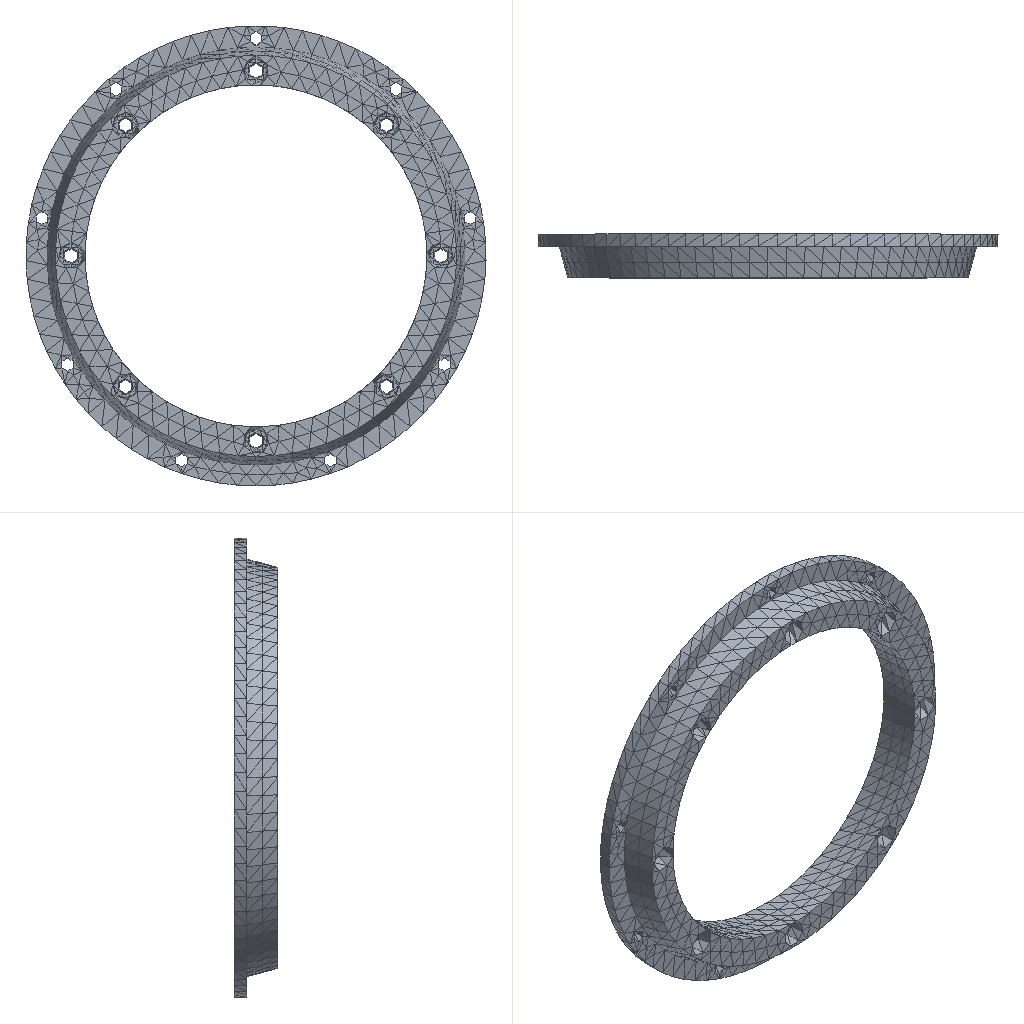Simulation study | nx simcenter
Set-up summary:
category,name,step,type,value,unit,region
solver,nx_nastran (Simcenter)
units,not stated in the deck,,not stated
analysis,deck,,static,static
analysis,solution,,SOL,101
load_step,SUBCASE 1,1,SUBCASE,SPC=1 LOAD=2
load_step,requested,,,1
mesh,nodes,,,9014
mesh,elements,,,4383
element_type,CTETRA,,solid,4383
load,nodal force total,,FX,0.0,model units
load,nodal force total,,FY,2499999.901,model units
load,nodal force total,,FZ,0.0,model units
load,load commands in deck,,count,543
bc,support commands in deck,,count,952
analysis,NX solution 0,,Structural,Linear Statics - Single Constraint
check,setup vs results,,match,every grid point's frame and coordinates and every element id; grid points of CTETRA elements
Nastran input file, long lists of numbers shortened:
$*$$$$$$$$$$$$$$$$$$$$$$$$$$$$$$$$$$$$$$$$$$$$$$$$$$$$$$$$$$$$$$$$$
$*
$*                    NX v10.0.0.24 TRANSLATOR
$*                    FOR NX NASTRAN VERSION 10.0
$ (33 more lines like these left out)
ASSIGN OUTPUT2='150_sim1-solution_1.op2' UNIT=12
$*
$*$$$$$$$$$$$$$$$$$$$$$$$$$$$$$$$$$$$
$*
$* EXECUTIVE CONTROL
$*
$*$$$$$$$$$$$$$$$$$$$$$$$$$$$$$$$$$$$
$*
ID,NASTRAN,150_sim1-solution_1
SOL 101
CEND
$*
$*$$$$$$$$$$$$$$$$$$$$$$$$$$$$$$$$$$$
$*
$* CASE CONTROL
$*
$*$$$$$$$$$$$$$$$$$$$$$$$$$$$$$$$$$$$
$*
TITLE = Solution 1
ECHO = NONE
SPC = 1
OUTPUT
BCRESULTS(TRACTION,FORCE,PLOT) = ALL
DISPLACEMENT(PLOT) = ALL
ESE(PLOT) = ALL
FORCE(PLOT,CORNER) = ALL
OLOAD(PLOT) = ALL
SPCFORCES(PLOT) = ALL
STRAIN(PLOT,FIBER,CORNER) = ALL
STRESS(PLOT,CORNER) = ALL
$*  NX Step: Subcase - Static Loads 1
SUBCASE 1
LABEL = Subcase - Static Loads 1
LOAD = 2
$*
$*$$$$$$$$$$$$$$$$$$$$$$$$$$$$$$$$$$$
$*
$* BULK DATA
$*
$*$$$$$$$$$$$$$$$$$$$$$$$$$$$$$$$$$$$
$*
BEGIN BULK
$*
$* PARAM CARDS
$*
PARAM      K6ROT100.0000
PARAM     OIBULK     YES
PARAM    OMACHPR     YES
PARAM       POST      -2
PARAM    POSTEXT     YES
PARAM    UNITSYS   MN-MM
$*
$* GRID CARDS
$*
GRID*               8936               0-6.893653870E+01-2.813807011E+00+
*       1.4255373001E+01               0
GRID*               8937               0-6.062178040E+01-2.813807011E+00+
*       -3.290000153E+01               0
$ (18024 more lines like these left out)
$*
$* ELEMENT CARDS
$*
$*  NX Mesh Collector: Solid(1)
$*  NX Mesh: 3d_mesh(1)
CTETRA         1       1       1       2       3    3976      80      81+
+             82      83      84      85
CTETRA         2       1       1       3    5059    5058      82      86+
+             87      88      89    6100
$ (8762 more lines like these left out)
$*
$* PROPERTY CARDS
$*
$*  NX Property: PSOLID1
PSOLID         1       1       0                           SMECH
$*
$* MATERIAL CARDS
$*
$*  NX Material: 3A21
MAT1           17.3119+7        0.3300002.7300-62.1355-5
MATT1          1       1               2               3
TABLEM1        1                                                        +
+        20.00007.3119+7 21.11007.3119+7 23.89007.3119+7 37.78007.3119+7+
+        51.67007.3119+7 65.56007.2429+7 79.44007.2429+7 93.33007.1739+7+
+       107.22007.1049+7121.11007.0359+7135.00006.9670+7148.89006.8980+7+
+       162.78006.8290+7176.67006.6910+7190.56006.6221+7204.44006.4841+7+
+       218.33006.3461+7232.22006.1392+7246.11006.0012+7260.00005.8633+7+
+       273.89005.7253+7287.78005.5184+7301.67005.3804+7315.56005.1735+7+
+       329.44004.9665+7343.33004.7596+7357.22004.6216+7371.11004.4147+7+
+           ENDT
TABLEM1        2                                                        +
+        20.00000.330000 21.11000.330000    ENDT
TABLEM1        3                                                        +
+        20.00002.1600-5 93.33002.2500-5107.22002.2662-5121.11002.2824-5+
+       135.00002.2968-5148.89002.3130-5162.78002.3274-5176.67002.3418-5+
+       190.56002.3544-5204.44002.3688-5218.33002.3814-5232.22002.3958-5+
+       246.11002.4066-5260.00002.4192-5273.89002.4300-5287.78002.4408-5+
+       301.67002.4498-5315.56002.4606-5329.44002.4696-5343.33002.4786-5+
+       357.22002.4876-5371.11002.4984-5385.00002.5110-5398.89002.5254-5+
+       412.78002.5398-5426.67002.5560-5    ENDT
$*
$* LOAD AND CONSTRAINT CARDS
$*
$*  NX Load and Constraint: Fixed(1)
SPC            1    3966  123456  0.0000
SPC            1    3967  123456  0.0000
SPC            1    3968  123456  0.0000
SPC            1    3969  123456  0.0000
$ (948 more lines like these left out)
$*  NX Load and Constraint: Force(1)
FORCE          2    3097       0 2518.46  0.00001.000000  0.0000
FORCE          2    3098       0985.1171  0.00001.000000  0.0000
FORCE          2    3099       0 3057.38  0.00001.000000  0.0000
FORCE          2    3100       0 4720.83  0.00001.000000  0.0000
$ (539 more lines like these left out)
ENDDATA 4d40d202
Results summary:
result,analysis,,,static
result,last_loadstep,,,1
result,primary field,,,displacements
result,reaction total,,FX,-0.04333,model units
result,reaction total,,FY,-2499999.0,model units
result,reaction total,,FZ,0.1309,model units
result,NX solution 0,,loadcases,1,mm